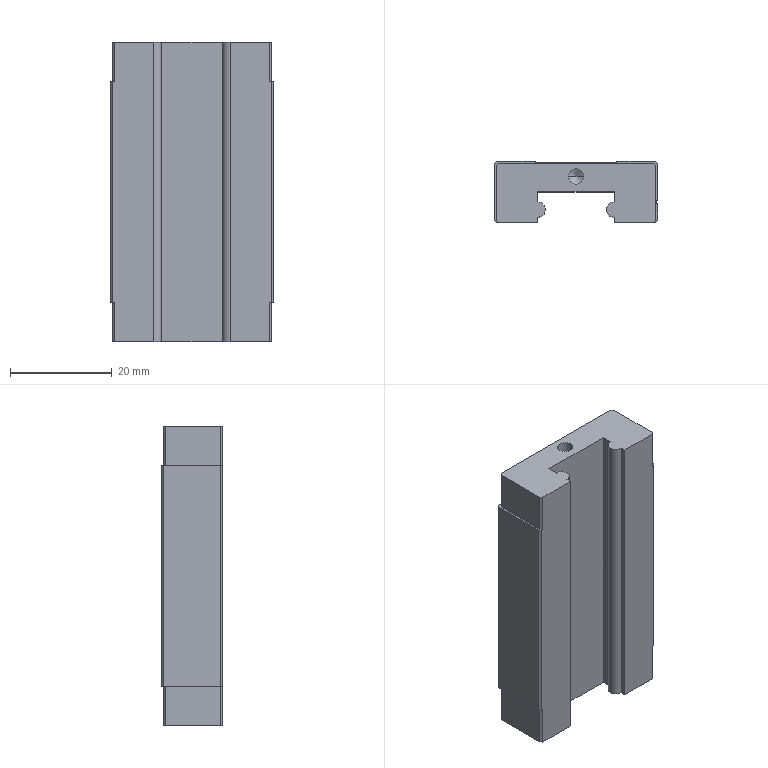Part | STEP file | 11-MANIFOLD_SOLID_BREP_3911 | 1 solid | 66 faces | box 32 x 12 x 58.8 mm | volume 16966 mm3 | plane 37 | cylinder 17 | cone 12 | commonest cylinder face diameters 3 x15 0.6 x2